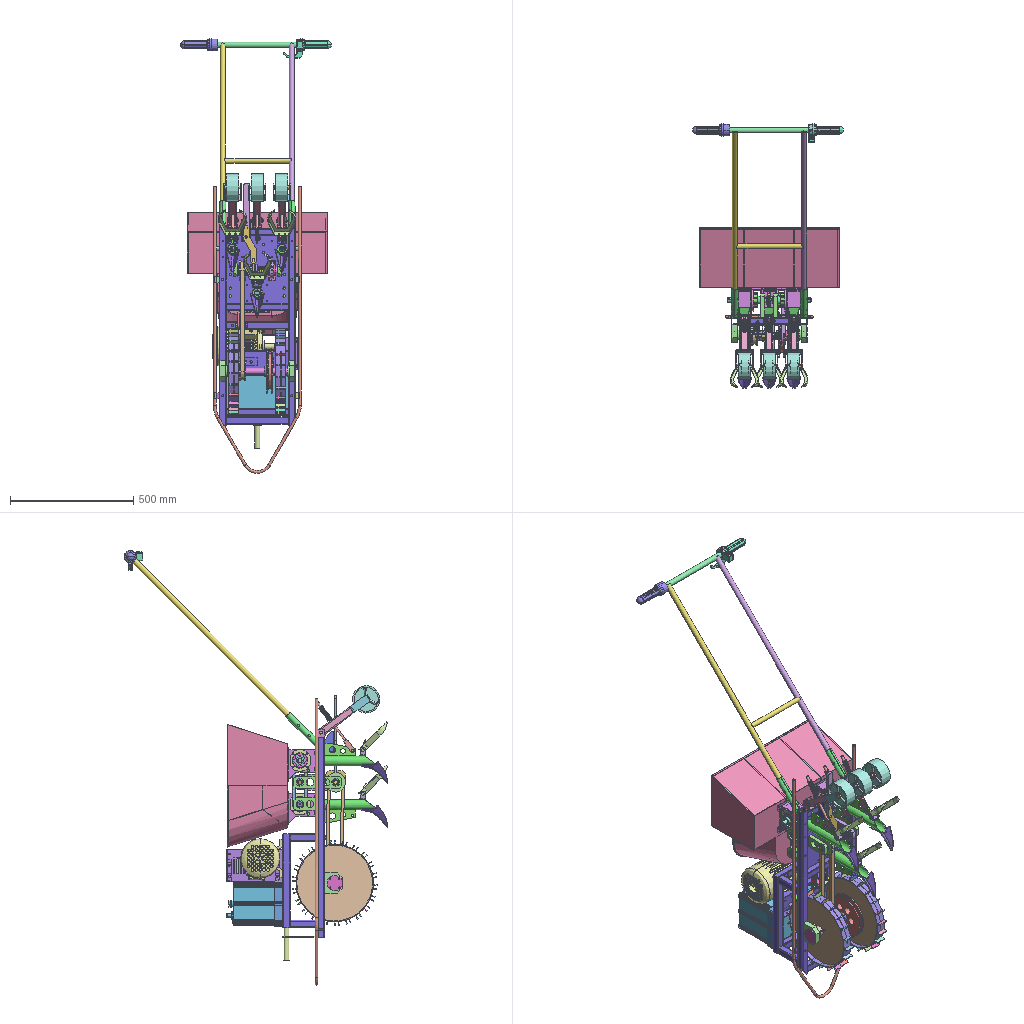Assembly | NX | 112 different items | 228 placed | box 612 x 1069 x 1762 mm
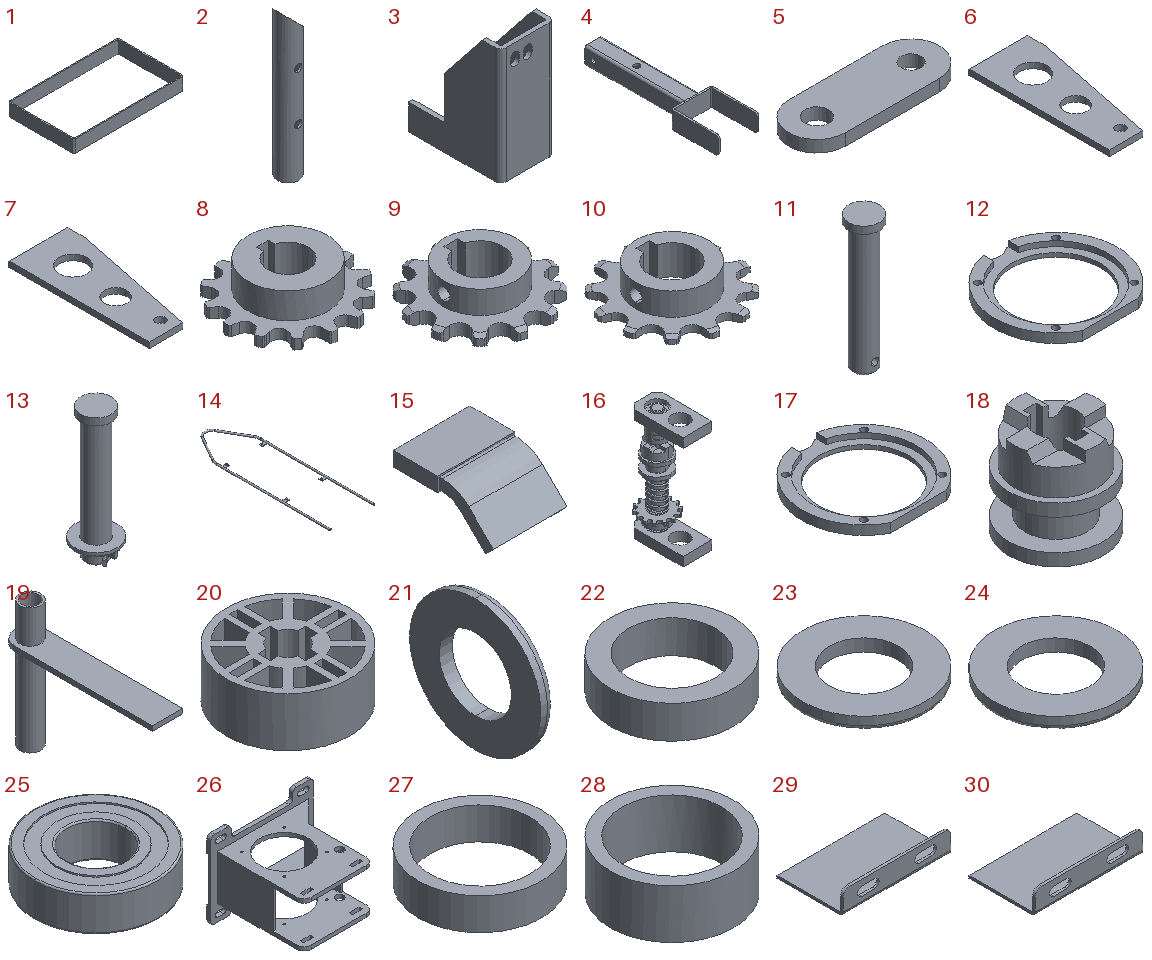Parts list (item | quantity | parent item | size | volume | features):
1 | x1 | in 99 | 306 x 182 x 35 mm | 100769 mm3 | features DATUM_CSYS 1, EXTRACT_DATUM_PLANE 1, EXTRUDE 1, SKETCH 1
2 | x1 | - | 26.5 x 26.5 x 180 mm | 30784 mm3 | features BREP 1
3 | x1 | in 99 | 38 x 65 x 82 mm | 28298 mm3 | features EXTRUDE 4, DATUM_CSYS 3, SKETCH 3, EXTRACT_DATUM_PLANE 1, UNITE 1
4 | x3 | in 99 | 71 x 253 x 30 mm | 87804 mm3 | features BLEND 2, DATUM_CSYS 2, EXTRACT_DATUM_PLANE 2, EXTRUDE 2, LINKED_BODY 2, SHELL 2, SKETCH 2, SUBTRACT 2
5 | x1 | in 40 | 64 x 24 x 5 mm | 6386 mm3 | features DATUM_CSYS 1, EXTRACT_DATUM_PLANE 1, EXTRUDE 1, SKETCH 1
6 | x3 | in 99 | 52 x 125 x 5 mm | 22141 mm3 | features DATUM_CSYS 1, EXTRACT_DATUM_PLANE 1, EXTRUDE 1, SKETCH 1
7 | x1 | - | 52 x 125 x 5 mm | 22141 mm3 | features DATUM_CSYS 1, EXTRACT_DATUM_PLANE 1, EXTRUDE 1, SKETCH 1
8 | x1 | in 16 | 61.9 x 60.843 x 18 mm | 22142 mm3 | features EXTRUDE 3, DATUM_CSYS 1, Delete Body 1, EXTRACT_DATUM_PLANE 1, SKETCH 1, UNITE 1
9 | x1 | in 58 | 52.696 x 52.696 x 15 mm | 11484 mm3 | features BREP 1
10 | x4 | in 58, 77, 85 | 52.696 x 52.696 x 13 mm | 8744 mm3 | features BREP 1
11 | x5 | in 13 | 11 x 11 x 47.5 mm | 2449 mm3 | features BREP 1
12 | x3 | in 77, 83, 84 | 89 x 83.264 x 6.6 mm | 13539 mm3 | features EXTRUDE 3, DATUM_CSYS 1, EXTRACT_DATUM_PLANE 1, SKETCH 1
13 | x5 | in 99 | 15 x 15.681 x 47.5 mm | 2690 mm3 | features BREP 2, BLEND 1, DATUM_CSYS 1, EXTRACT_DATUM_PLANE 1, EXTRUDE 1, SKETCH 1
14 | x1 | in 99 | 356.002 x 1162 x 12 mm | 288211 mm3 | features DATUM_CSYS 1, DATUM_PLANE 1, EXTRUDE 1, SKETCH 1, SWP104 1
15 | x2 | in 83, 84 | 48 x 61.688 x 28.188 mm | 24699 mm3 | features EXTRUDE 2, DATUM_CSYS 1, LINKED_FACE 1, SKETCH 1, UNITE 1
16 | x1 | in 99 | 60.843 x 100.95 x 194.5 mm | 245007 mm3 | features EXTRUDE 9, DATUM_CSYS 7, EXTRACT_DATUM_PLANE 7, SKETCH 7, BREP 4, UNITE 2, CHAMFER 1, Delete Body 1
17 | x1 | - | 89 x 83.264 x 6.6 mm | 13539 mm3 | features EXTRUDE 3, DATUM_CSYS 1, EXTRACT_DATUM_PLANE 1, SKETCH 1
18 | x1 | in 16 | 46 x 46 x 45 mm | 34964 mm3 | features BREP 1, DATUM_CSYS 1, EXTRACT_DATUM_PLANE 1, SKETCH 1
19 | x1 | in 99 | 32 x 161 x 132.5 mm | 39960 mm3 | features EXTRUDE 3, DATUM_CSYS 1, EXTRACT_DATUM_PLANE 1, SKETCH 1, UNITE 1
20 | x3 | in 77, 83, 84 | 60.7 x 60.7 x 24.4 mm | 36264 mm3 | features DATUM_CSYS 1, EXTRUDE 1, LINKED_FACE 1, SKETCH 1
21 | x3 | in 44 | 2 x 20 x 20 mm | 425.07 mm3 | features BREP 1
22 | x2 | in 40 | 15 x 15 x 4 mm | 360.498 mm3 | features DATUM_CSYS 1, EXTRACT_DATUM_PLANE 1, EXTRUDE 1, SKETCH 1
23 | x3 | in 92 | 15 x 15 x 1.5 mm | 179.214 mm3 | features BREP 1
24 | x5 | in 13 | 15 x 15 x 1.5 mm | 179.214 mm3 | features BLEND 1, DATUM_CSYS 1, EXTRACT_DATUM_PLANE 1, EXTRUDE 1, SKETCH 1
25 | x2 | in 99 | 42 x 42 x 12 mm | 12431 mm3 | features BREP 1
26 | x3 | in 77, 83, 84 | 136.5 x 120 x 103 mm | 129475 mm3 | features DATUM_CSYS 2, EXTRUDE 2, SKETCH 2, BREP 1, EXTRACT_DATUM_PLANE 1, INTERSECT 1, UNITE 1
27 | x3 | in 16, 85 | 25 x 25 x 6.5 mm | 1108 mm3 | features DATUM_CSYS 1, EXTRACT_DATUM_PLANE 1, EXTRUDE 1, SKETCH 1
28 | x2 | in 16, 85 | 25 x 25 x 10 mm | 1704 mm3 | features DATUM_CSYS 1, EXTRACT_DATUM_PLANE 1, EXTRUDE 1, SKETCH 1
29 | x2 | in 61 | 85 x 52 x 18 mm | 10959 mm3 | features BLEND 2, DATUM_CSYS 2, EXTRUDE 2, SKETCH 2, EXTRACT_DATUM_PLANE 1
30 | x1 | - | 85 x 52 x 18 mm | 10959 mm3 | features BLEND 2, DATUM_CSYS 2, EXTRUDE 2, SKETCH 2, EXTRACT_DATUM_PLANE 1
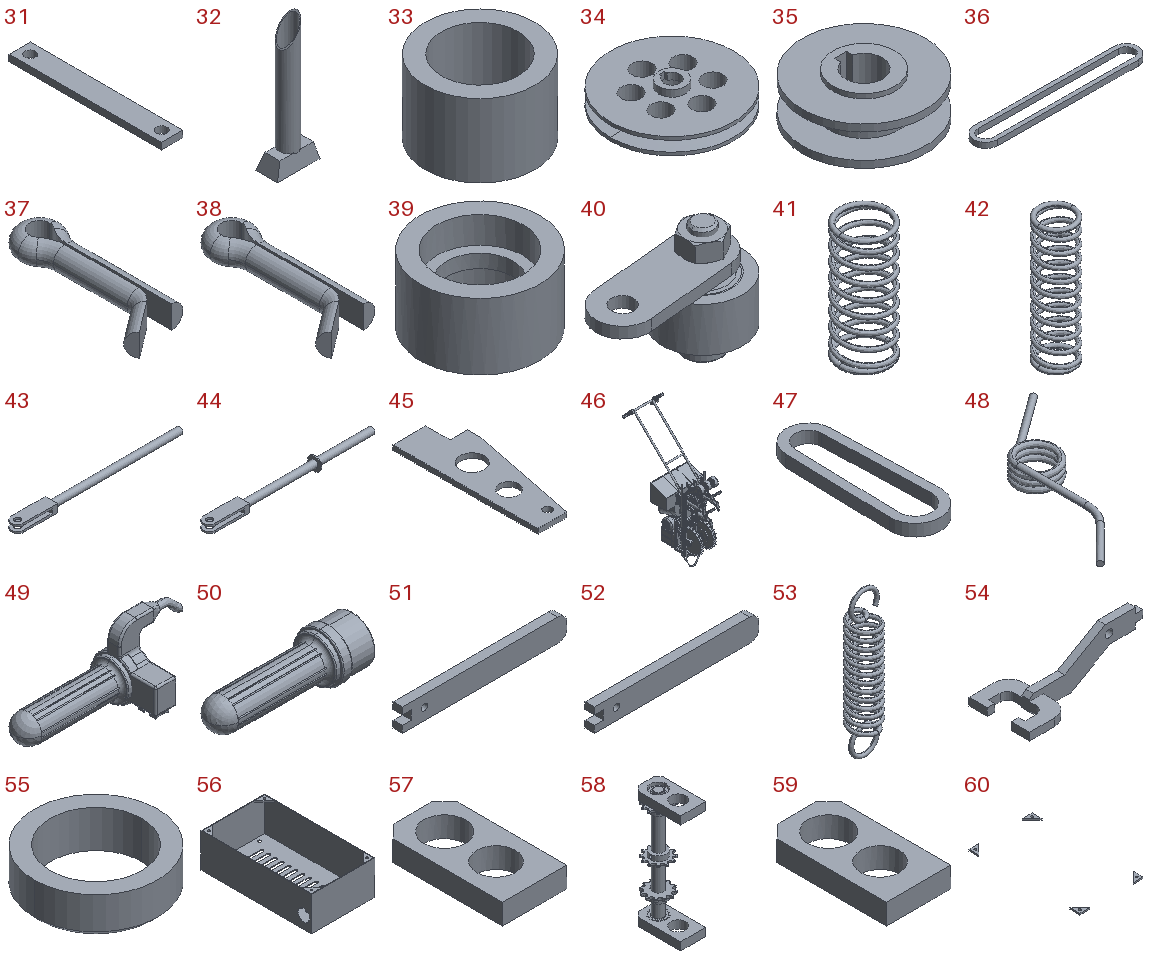31 | x6 | in 77, 83, 84 | 13 x 93 x 4 mm | 4571 mm3 | features EXTRUDE 2, DATUM_CSYS 1, EXTRACT_DATUM_PLANE 1, SKETCH 1
32 | x3 | in 99 | 95 x 48 x 289.397 mm | 75187 mm3 | features EXTRUDE 4, DATUM_CSYS 3, SKETCH 3, EXTRACT_DATUM_PLANE 2, SHELL 2, DRAFT 1, UNITE 1
33 | x5 | in 99 | 15 x 15 x 10 mm | 901.244 mm3 | features DATUM_CSYS 1, EXTRACT_DATUM_PLANE 1, EXTRUDE 1, SKETCH 1
34 | x1 | in 99 | 185 x 185 x 35 mm | 385967 mm3 | features EXTRUDE 2, BREP 1, DATUM_CSYS 1, EXTRACT_DATUM_PLANE 1, INTERSECT 1, SKETCH 1
35 | x2 | in 46, 99 | 80 x 80 x 28 mm | 60999 mm3 | features EXTRUDE 3, DATUM_CSYS 1, LINKED_FACE 1, SKETCH 1, UNITE 1
36 | x1 | in 99 | 477.82 x 73.07 x 16 mm | 191391 mm3 | features DATUM_CSYS 1, EXTRUDE 1, LINKED_FACE 1, SKETCH 1
37 | x5 | in 13 | 6.586 x 15.587 x 2.2 mm | 61.721 mm3 | features BREP 1
38 | x3 | in 92 | 6.586 x 15.587 x 2.2 mm | 61.721 mm3 | features BREP 1
39 | x1 | in 40 | 36 x 36 x 20 mm | 10606 mm3 | features EXTRUDE 2, DATUM_CSYS 1, EXTRACT_DATUM_PLANE 1, SKETCH 1, UNITE 1
40 | x1 | in 99 | 69.825 x 36 x 50 mm | 31125 mm3 | features EXTRUDE 4, BREP 3, DATUM_CSYS 3, EXTRACT_DATUM_PLANE 3, SKETCH 3, UNITE 1
41 | x1 | in 16 | 28.5 x 28.5 x 66.5 mm | 3897 mm3 | features BREP 1
42 | x3 | in 99 | 18 x 18 x 62 mm | 1869 mm3 | features BREP 1
43 | x3 | in 44 | 249 x 18 x 12 mm | 21761 mm3 | features EXTRUDE 3, DATUM_CSYS 2, SKETCH 1, SWP104 1, UNITE 1
44 | x3 | in 99 | 249 x 20 x 20 mm | 22186 mm3 | features EXTRUDE 3, DATUM_CSYS 2, BREP 1, SKETCH 1, SWP104 1, UNITE 1
45 | x1 | in 99 | 52 x 150 x 5 mm | 26391 mm3 | features DATUM_CSYS 1, EXTRACT_DATUM_PLANE 1, EXTRUDE 1, SKETCH 1
46 | x1 | - | - | 25576311 mm3 | features EXTRUDE 114, DATUM_CSYS 75, SKETCH 74, EXTRACT_DATUM_PLANE 45, BREP 36, EXTRACT_BODY 25, UNITE 18, LINKED_FACE 16, BLEND 10, LINKED_BODY 5, SHELL 5, CHAMFER 4, SUBTRACT 4, SWP104 4, INTERSECT 3, DATUM_PLANE 2, Delete Body 2, EXTRACT_STRING 2, Pattern Geometry 2, Container 1, DRAFT 1, Geometry Instance 1, HOLE PACKAGE 1, Instance Feature 1, MOVE_FACE 1, Mirror Feature 1, OFFSET 1, REPLACE_FACE 1, SCALE 1, SIMPLE HOLE 1, SYMBOLIC_THREAD 1
47 | x1 | in 99 | 69.07 x 210.07 x 16 mm | 87712 mm3 | features DATUM_CSYS 1, EXTRUDE 1, LINKED_FACE 1, SKETCH 1
48 | x3 | in 99 | 41.247 x 61.989 x 7.45 mm | 454.454 mm3 | features BREP 1
49 | x1 | in 99 | 194.399 x 75 x 80 mm | 130735 mm3 | features BREP 1
50 | x1 | in 99 | 151 x 50 x 50 mm | 105394 mm3 | features BREP 1
51 | x1 | in 99 | 180.75 x 10 x 25 mm | 43395 mm3 | features DATUM_CSYS 1, EXTRACT_DATUM_PLANE 1, EXTRUDE 1, SKETCH 1
52 | x1 | - | 180.75 x 10 x 25 mm | 43395 mm3 | features DATUM_CSYS 1, EXTRACT_DATUM_PLANE 1, EXTRUDE 1, SKETCH 1
53 | x1 | in 99 | 16 x 16 x 80 mm | 1981 mm3 | features BREP 1
54 | x1 | in 99 | 185 x 80 x 55 mm | 60646 mm3 | features DATUM_CSYS 2, EXTRUDE 2, SKETCH 2, EXTRACT_DATUM_PLANE 1, LINKED_FACE 1
55 | x2 | in 86 | 23 x 23 x 7 mm | 1284 mm3 | features BREP 1
56 | x1 | in 99 | 130 x 226 x 70 mm | 110866 mm3 | features EXTRUDE 4, DATUM_CSYS 3, SKETCH 3, EXTRACT_DATUM_PLANE 1, LINKED_FACE 1
57 | x8 | in 16, 58, 77, 85 | 50 x 95 x 16 mm | 50222 mm3 | features DATUM_CSYS 1, EXTRACT_DATUM_PLANE 1, EXTRUDE 1, SKETCH 1
58 | x1 | in 99 | 53.723 x 96.862 x 234.5 mm | 212399 mm3 | features BREP 4, DATUM_CSYS 1, EXTRACT_DATUM_PLANE 1, EXTRUDE 1, SKETCH 1
59 | x1 | - | 50 x 95 x 16 mm | 50222 mm3 | features DATUM_CSYS 1, EXTRACT_DATUM_PLANE 1, EXTRUDE 1, SKETCH 1
60 | x1 | in 56 | 127 x 223 x 3 mm | 2234 mm3 | features DATUM_CSYS 1, EXTRACT_DATUM_PLANE 1, EXTRUDE 1, SKETCH 1
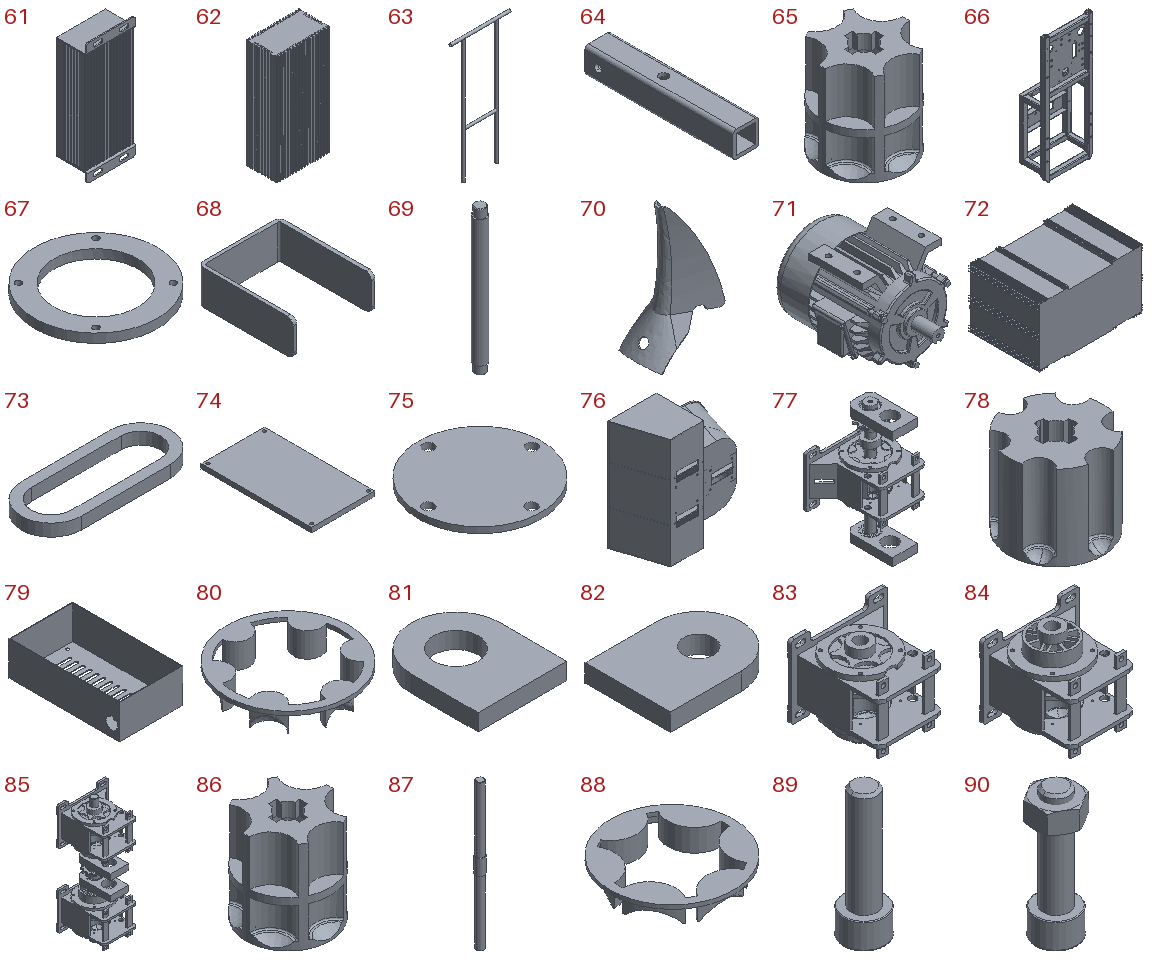61 | x1 | in 99 | 85 x 52 x 210 mm | 665220 mm3 | features DATUM_CSYS 3, EXTRUDE 3, SKETCH 3, BLEND 2, EXTRACT_DATUM_PLANE 2
62 | x1 | in 61 | 85 x 50 x 174 mm | 643303 mm3 | features DATUM_CSYS 1, EXTRACT_DATUM_PLANE 1, EXTRUDE 1, SKETCH 1
63 | x1 | in 99 | 500 x 21.5 x 1061 mm | 830822 mm3 | features EXTRACT_DATUM_PLANE 4, DATUM_CSYS 3, SKETCH 3, EXTRUDE 2, Container 1, EXTRACT_BODY 1, Geometry Instance 1, MOVE_FACE 1, SWP104 1, UNITE 1
64 | x3 | in 4 | - | 67348 mm3 | features LINKED_BODY 2, SUBTRACT 2, BLEND 1, DATUM_CSYS 1, EXTRACT_DATUM_PLANE 1, EXTRUDE 1, SHELL 1, SKETCH 1
65 | x2 | in 86 | 60.7 x 60.7 x 66.6 mm | 88337 mm3 | features BREP 1
66 | x1 | in 99 | 310 x 170 x 810 mm | 1667503 mm3 | features BREP 1, DATUM_CSYS 1, EXTRACT_DATUM_PLANE 1, SKETCH 1
67 | x3 | in 77, 83, 84 | 90 x 90 x 6.5 mm | 21817 mm3 | features DATUM_CSYS 1, EXTRUDE 1, LINKED_FACE 1, SKETCH 1
68 | x3 | in 4 | 71 x 83 x 30 mm | 20455 mm3 | features BLEND 1, DATUM_CSYS 1, EXTRACT_DATUM_PLANE 1, EXTRUDE 1, SHELL 1, SKETCH 1
69 | x1 | in 58 | 20 x 20 x 231.5 mm | 68985 mm3 | features BREP 1
70 | x3 | in 99 | 60.225 x 56.002 x 125 mm | 14163 mm3 | features BREP 1
71 | x1 | in 46 | - | 2573797 mm3 | features BREP 1, HOLE PACKAGE 1, OFFSET 1, SCALE 1, SIMPLE HOLE 1, SYMBOLIC_THREAD 1
72 | x1 | in 46 | 304 x 227 x 174.5 mm | 9929368 mm3 | features EXTRUDE 10, BLEND 2, DATUM_CSYS 2, SKETCH 2, EXTRACT_DATUM_PLANE 1, UNITE 1
73 | x2 | in 99 | 147.5 x 59 x 12 mm | 79425 mm3 | features BREP 1, DATUM_CSYS 1, EXTRACT_DATUM_PLANE 1, EXTRUDE 1, SKETCH 1
74 | x1 | in 99 | 128 x 224 x 9.5 mm | 271310 mm3 | features DATUM_CSYS 1, EXTRACT_DATUM_PLANE 1, EXTRUDE 1, SKETCH 1
75 | x2 | in 99 | 62 x 62 x 3 mm | 8772 mm3 | features DATUM_CSYS 1, EXTRUDE 1, LINKED_FACE 1, SKETCH 1
76 | x1 | in 99 | 499.609 x 244.468 x 567.002 mm | 2802916 mm3 | features DATUM_CSYS 2, SKETCH 2, BREP 1, LINKED_FACE 1
77 | x1 | in 99 | 136.5 x 120 x 240 mm | 520040 mm3 | features EXTRUDE 21, DATUM_CSYS 11, SKETCH 11, LINKED_FACE 6, BREP 5, UNITE 5, EXTRACT_DATUM_PLANE 4, EXTRACT_BODY 3, CHAMFER 2, INTERSECT 2, LINKED_BODY 1, Pattern Geometry 1, REPLACE_FACE 1
78 | x1 | in 77 | 60.7 x 60.7 x 55 mm | 113119 mm3 | features EXTRUDE 2, BREP 1, DATUM_CSYS 1, INTERSECT 1, LINKED_BODY 1, LINKED_FACE 1, SKETCH 1, UNITE 1
79 | x1 | in 56 | 130 x 226 x 70 mm | 108632 mm3 | features EXTRUDE 3, DATUM_CSYS 2, SKETCH 2, LINKED_FACE 1
80 | x1 | in 77 | 70 x 70 x 14 mm | 7900 mm3 | features BREP 1
81 | x2 | in 99 | 16 x 20 x 3 mm | 726.796 mm3 | features DATUM_CSYS 1, EXTRACT_DATUM_PLANE 1, EXTRUDE 1, SKETCH 1
82 | x1 | in 99 | 32 x 24 x 5 mm | 3247 mm3 | features DATUM_CSYS 1, EXTRUDE 1, LINKED_FACE 1, SKETCH 1
83 | x1 | in 85 | 136.5 x 120 x 117.9 mm | 352197 mm3 | features EXTRUDE 14, DATUM_CSYS 8, SKETCH 8, BREP 4, LINKED_FACE 4, EXTRACT_BODY 3, EXTRACT_DATUM_PLANE 3, UNITE 3, INTERSECT 1, Pattern Geometry 1, REPLACE_FACE 1
84 | x1 | in 85 | 136.5 x 120 x 117.9 mm | 352197 mm3 | features EXTRUDE 14, DATUM_CSYS 8, SKETCH 8, BREP 4, LINKED_FACE 4, EXTRACT_BODY 3, EXTRACT_DATUM_PLANE 3, UNITE 3, INTERSECT 1, Pattern Geometry 1, REPLACE_FACE 1
85 | x1 | in 99 | 136.5 x 120 x 340 mm | 908883 mm3 | features EXTRUDE 18, DATUM_CSYS 12, SKETCH 12, BREP 7, EXTRACT_DATUM_PLANE 6, LINKED_FACE 4, EXTRACT_BODY 3, UNITE 3, DATUM_PLANE 1, Delete Body 1, INTERSECT 1, Pattern Geometry 1, REPLACE_FACE 1
86 | x2 | in 83, 84 | 60.7 x 60.7 x 66.6 mm | 89622 mm3 | features BREP 2
87 | x1 | in 85 | 20 x 20 x 340 mm | 77391 mm3 | features BREP 1, DATUM_CSYS 1, DATUM_PLANE 1, Delete Body 1, EXTRUDE 1, SKETCH 1
88 | x2 | in 83, 84 | 70 x 70 x 12.6 mm | 14086 mm3 | features BREP 1
89 | x1 | in 90 | 16 x 16 x 50 mm | 4800 mm3 | features BREP 1
90 | x1 | in 40 | 16 x 18.475 x 50 mm | 6567 mm3 | features BREP 2
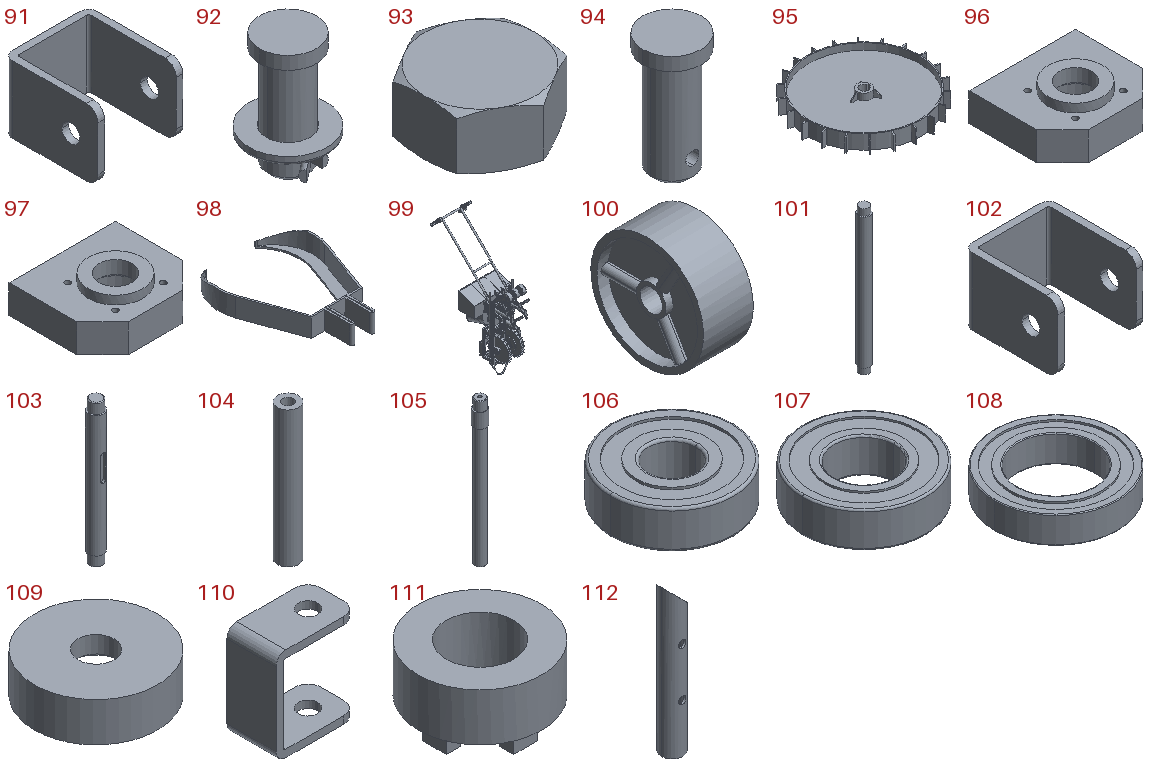91 | x3 | in 99 | - | 9881 mm3 | features BLEND 1, DATUM_CSYS 1, EXTRACT_DATUM_PLANE 1, EXTRUDE 1, LINKED_BODY 1, SKETCH 1, SUBTRACT 1
92 | x3 | in 99 | 15 x 15.681 x 22.5 mm | 1434 mm3 | features BREP 3
93 | x1 | in 90 | 16 x 18.475 x 8 mm | 1767 mm3 | features BREP 1
94 | x3 | in 92 | 11 x 11 x 22.5 mm | 1193 mm3 | features BREP 1
95 | x2 | in 99 | 344.986 x 341.901 x 40 mm | 408899 mm3 | features EXTRACT_BODY 21, EXTRUDE 5, CHAMFER 1, DATUM_CSYS 1, EXTRACT_DATUM_PLANE 1, Pattern Geometry 1, SKETCH 1, UNITE 1
96 | x2 | in 99 | 82 x 72 x 28.5 mm | 96953 mm3 | features EXTRUDE 7, DATUM_CSYS 2, SKETCH 2, LINKED_FACE 1
97 | x1 | - | 82 x 72 x 28.5 mm | 96953 mm3 | features EXTRUDE 7, DATUM_CSYS 2, SKETCH 2, LINKED_FACE 1
98 | x3 | in 99 | 113.914 x 159.253 x 22 mm | 25744 mm3 | features EXTRUDE 3, DATUM_CSYS 2, EXTRACT_STRING 2, SKETCH 2, Instance Feature 1, Mirror Feature 1, SHELL 1
99 | x1 | in 46 | - | 13012932 mm3 | features EXTRUDE 104, DATUM_CSYS 73, SKETCH 72, EXTRACT_DATUM_PLANE 44, BREP 35, EXTRACT_BODY 25, UNITE 17, LINKED_FACE 16, BLEND 8, LINKED_BODY 5, SHELL 5, CHAMFER 4, SUBTRACT 4, SWP104 4, INTERSECT 3, DATUM_PLANE 2, Delete Body 2, EXTRACT_STRING 2, Pattern Geometry 2, Container 1, DRAFT 1, Geometry Instance 1, Instance Feature 1, MOVE_FACE 1, Mirror Feature 1, REPLACE_FACE 1
100 | x3 | in 99 | 49 x 111 x 111 mm | 318902 mm3 | features EXTRUDE 3, BLEND 1, DATUM_CSYS 1, EXTRACT_DATUM_PLANE 1, SKETCH 1, UNITE 1
101 | x1 | in 99 | 23.908 x 23.908 x 299 mm | 125501 mm3 | features DATUM_CSYS 1, EXTRACT_DATUM_PLANE 1, EXTRUDE 1, SKETCH 1, SWP104 1
102 | x1 | - | 38 x 42 x 30 mm | 9881 mm3 | features BLEND 1, DATUM_CSYS 1, EXTRACT_DATUM_PLANE 1, EXTRUDE 1, LINKED_BODY 1, SKETCH 1, SUBTRACT 1
103 | x1 | in 16 | 20 x 20 x 191.953 mm | 57075 mm3 | features EXTRUDE 3, DATUM_CSYS 2, EXTRACT_DATUM_PLANE 2, SKETCH 2, CHAMFER 1, UNITE 1
104 | x3 | in 99 | 10 x 10 x 65 mm | 3829 mm3 | features DATUM_CSYS 1, EXTRACT_DATUM_PLANE 1, EXTRUDE 1, SKETCH 1
105 | x1 | in 77 | 20 x 20 x 233 mm | 50412 mm3 | features EXTRUDE 4, CHAMFER 2, DATUM_CSYS 1, LINKED_FACE 1, SKETCH 1, UNITE 1
106 | x2 | in 40 | 26 x 26 x 8 mm | 3423 mm3 | features BREP 1
107 | x8 | in 16, 58, 77, 85 | 35 x 35 x 10 mm | 6999 mm3 | features BREP 1
108 | x3 | in 16 | 32 x 32 x 7 mm | 3226 mm3 | features BREP 1
109 | x1 | in 77 | 22 x 22 x 7 mm | 1632 mm3 | features EXTRUDE 2, DATUM_CSYS 1, LINKED_FACE 1, SKETCH 1, UNITE 1
110 | x3 | in 99 | 33 x 20 x 38 mm | 5372 mm3 | features BLEND 1, DATUM_CSYS 1, EXTRACT_DATUM_PLANE 1, EXTRUDE 1, LINKED_BODY 1, SKETCH 1, SUBTRACT 1
111 | x6 | in 77, 83, 84 | 31 x 31 x 17.802 mm | 6776 mm3 | features EXTRACT_BODY 3, EXTRUDE 3, DATUM_CSYS 1, LINKED_FACE 1, Pattern Geometry 1, REPLACE_FACE 1, SKETCH 1, UNITE 1
112 | x2 | in 99 | 26.5 x 26.5 x 180 mm | 30784 mm3 | features BREP 1
Mates (type | each side: item.copy, entity, surface, feature):
In subassembly 46
Touch | 71.1 face plane Body(1) | 66.1 face plane Body(0)
In subassembly 99
Touch | 101.1 | 34.1
Fix | 66.1 component